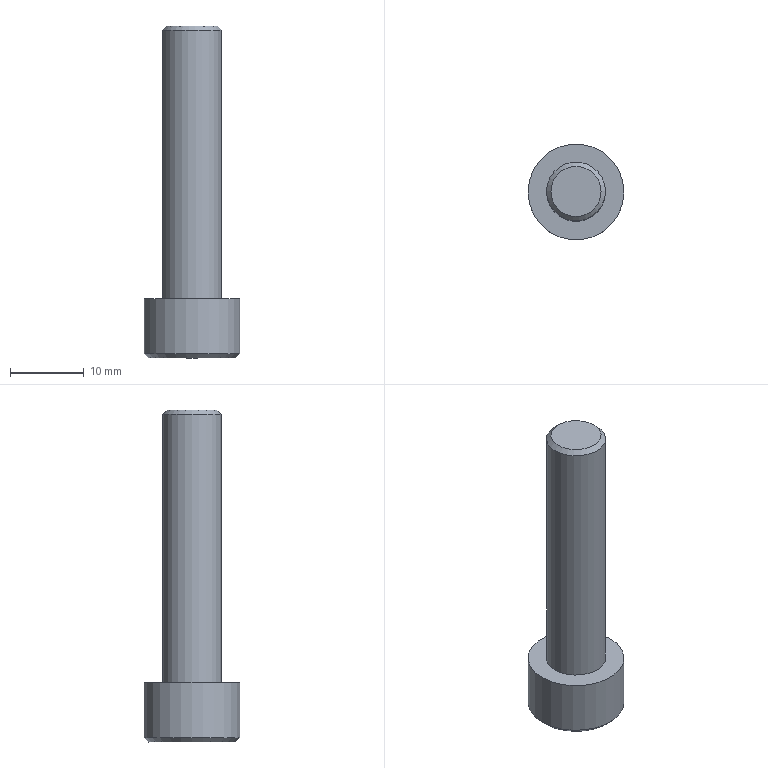Part | STEP file | solid 18 | 1 solid | 14 faces | box 13 x 13 x 45 mm | volume 2786 mm3 | plane 10 | cone 2 | cylinder 2 | commonest cylinder face diameters 8 x1 13 x1